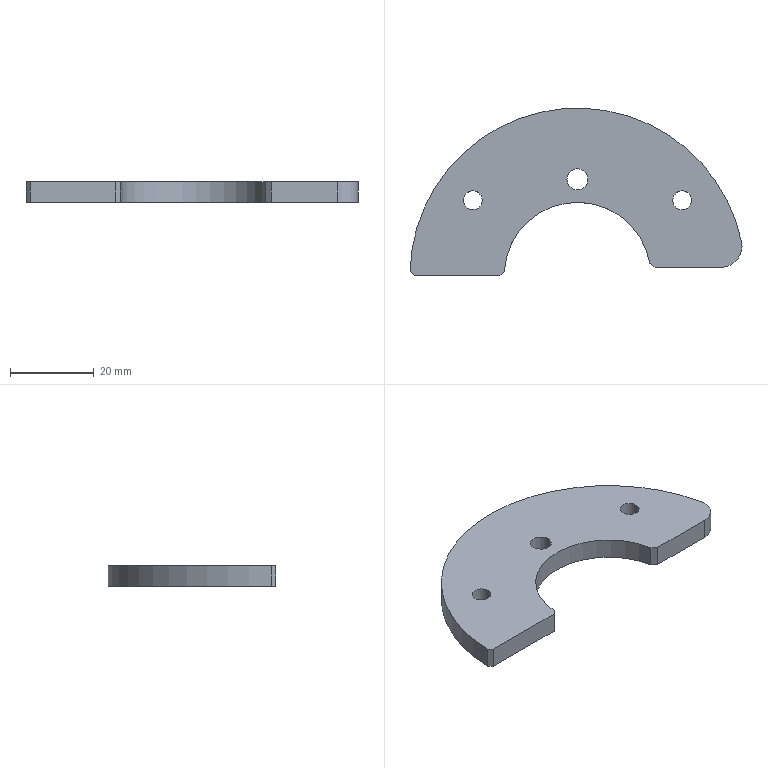Part | STEP file | End cover plate-upper | 1 solid | 16 faces | box 79.281 x 40 x 5 mm | volume 9633 mm3 | cylinder 9 | plane 7 | commonest cylinder face diameters 4.5 x4 5 x2 10 x1 35 x1 80 x1
STEP:
#1=CARTESIAN_POINT('',(0.,0.,0.));
#2=DIRECTION('',(0.,0.,1.));
#3=DIRECTION('',(1.,0.,0.));
#4=AXIS2_PLACEMENT_3D('',#1,#2,#3);
#5=CARTESIAN_POINT('',(-22.75,18.,0.));
#6=VERTEX_POINT('',#5);
#7=CARTESIAN_POINT('',(-22.75,18.,5.));
#8=VERTEX_POINT('',#7);
#9=CARTESIAN_POINT('',(-22.75,18.,5.));
#10=DIRECTION('',(0.,0.,1.));
#11=VECTOR('',#10,1.);
#12=LINE('',#9,#11);
#13=CARTESIAN_POINT('',(-25.,18.,5.));
#14=DIRECTION('',(0.,0.,1.));
#15=DIRECTION('',(1.,0.,0.));
#16=AXIS2_PLACEMENT_3D('',#13,#14,#15);
#17=CYLINDRICAL_SURFACE('',#16,2.25);
#18=CARTESIAN_POINT('',(6.283,0.));
#19=DIRECTION('',(0.,1.));
#20=VECTOR('',#19,1.);
#21=LINE('',#18,#20);
#22=(GEOMETRIC_REPRESENTATION_CONTEXT(2)PARAMETRIC_REPRESENTATION_CONTEXT()REPRESENTATION_CONTEXT('',''));
#23=DEFINITIONAL_REPRESENTATION('',(#21),#22);
#24=PCURVE('',#17,#23);
#25=CARTESIAN_POINT('',(-25.,18.,5.));
#26=DIRECTION('',(0.,0.,1.));
#27=DIRECTION('',(1.,0.,0.));
#28=AXIS2_PLACEMENT_3D('',#25,#26,#27);
#29=CYLINDRICAL_SURFACE('',#28,2.25);
#30=CARTESIAN_POINT('',(0.,0.));
#31=DIRECTION('',(0.,1.));
#32=VECTOR('',#31,1.);
#33=LINE('',#30,#32);
#34=(GEOMETRIC_REPRESENTATION_CONTEXT(2)PARAMETRIC_REPRESENTATION_CONTEXT()REPRESENTATION_CONTEXT('',''));
#35=DEFINITIONAL_REPRESENTATION('',(#33),#34);
#36=PCURVE('',#29,#35);
#37=SURFACE_CURVE('',#12,(#24,#36),.PCURVE_S1.);
#38=EDGE_CURVE('',#6,#8,#37,.T.);
#39=ORIENTED_EDGE('',*,*,#38,.T.);
#40=CARTESIAN_POINT('',(-27.25,18.,5.));
#41=VERTEX_POINT('',#40);
#42=CARTESIAN_POINT('',(-25.,18.,5.));
#43=DIRECTION('',(0.,0.,1.));
#44=DIRECTION('',(1.,0.,0.));
#45=AXIS2_PLACEMENT_3D('',#42,#43,#44);
#46=CIRCLE('',#45,2.25);
#47=CARTESIAN_POINT('',(0.,0.));
#48=DIRECTION('',(1.,0.));
#49=VECTOR('',#48,1.);
#50=LINE('',#47,#49);
#51=(GEOMETRIC_REPRESENTATION_CONTEXT(2)PARAMETRIC_REPRESENTATION_CONTEXT()REPRESENTATION_CONTEXT('',''));
#52=DEFINITIONAL_REPRESENTATION('',(#50),#51);
#53=PCURVE('',#17,#52);
#54=CARTESIAN_POINT('',(0.,0.,5.));
#55=DIRECTION('',(0.,0.,1.));
#56=DIRECTION('',(1.,0.,0.));
#57=AXIS2_PLACEMENT_3D('',#54,#55,#56);
#58=PLANE('',#57);
#59=CARTESIAN_POINT('',(-25.,18.));
#60=DIRECTION('',(1.,0.));
#61=AXIS2_PLACEMENT_2D('',#59,#60);
#62=CIRCLE('',#61,2.25);
#63=(GEOMETRIC_REPRESENTATION_CONTEXT(2)PARAMETRIC_REPRESENTATION_CONTEXT()REPRESENTATION_CONTEXT('',''));
#64=DEFINITIONAL_REPRESENTATION('',(#62),#63);
#65=PCURVE('',#58,#64);
#66=SURFACE_CURVE('',#46,(#53,#65),.PCURVE_S1.);
#67=EDGE_CURVE('',#41,#8,#66,.T.);
#68=ORIENTED_EDGE('',*,*,#67,.F.);
#69=CARTESIAN_POINT('',(-27.25,18.,0.));
#70=VERTEX_POINT('',#69);
#71=CARTESIAN_POINT('',(-27.25,18.,5.));
#72=DIRECTION('',(0.,0.,1.));
#73=VECTOR('',#72,1.);
#74=LINE('',#71,#73);
#75=CARTESIAN_POINT('',(3.142,0.));
#76=DIRECTION('',(0.,1.));
#77=VECTOR('',#76,1.);
#78=LINE('',#75,#77);
#79=(GEOMETRIC_REPRESENTATION_CONTEXT(2)PARAMETRIC_REPRESENTATION_CONTEXT()REPRESENTATION_CONTEXT('',''));
#80=DEFINITIONAL_REPRESENTATION('',(#78),#79);
#81=PCURVE('',#17,#80);
#82=CARTESIAN_POINT('',(3.142,0.));
#83=DIRECTION('',(0.,1.));
#84=VECTOR('',#83,1.);
#85=LINE('',#82,#84);
#86=(GEOMETRIC_REPRESENTATION_CONTEXT(2)PARAMETRIC_REPRESENTATION_CONTEXT()REPRESENTATION_CONTEXT('',''));
#87=DEFINITIONAL_REPRESENTATION('',(#85),#86);
#88=PCURVE('',#29,#87);
#89=SURFACE_CURVE('',#74,(#81,#88),.PCURVE_S1.);
#90=EDGE_CURVE('',#70,#41,#89,.T.);
#91=ORIENTED_EDGE('',*,*,#90,.F.);
#92=CARTESIAN_POINT('',(-25.,18.,0.));
#93=DIRECTION('',(0.,0.,1.));
#94=DIRECTION('',(1.,0.,0.));
#95=AXIS2_PLACEMENT_3D('',#92,#93,#94);
#96=CIRCLE('',#95,2.25);
#97=CARTESIAN_POINT('',(0.,-5.));
#98=DIRECTION('',(1.,0.));
#99=VECTOR('',#98,1.);
#100=LINE('',#97,#99);
#101=(GEOMETRIC_REPRESENTATION_CONTEXT(2)PARAMETRIC_REPRESENTATION_CONTEXT()REPRESENTATION_CONTEXT('',''));
#102=DEFINITIONAL_REPRESENTATION('',(#100),#101);
#103=PCURVE('',#17,#102);
#104=CARTESIAN_POINT('',(0.,0.,0.));
#105=DIRECTION('',(0.,0.,1.));
#106=DIRECTION('',(1.,0.,0.));
#107=AXIS2_PLACEMENT_3D('',#104,#105,#106);
#108=PLANE('',#107);
#109=CARTESIAN_POINT('',(-25.,18.));
#110=DIRECTION('',(1.,0.));
#111=AXIS2_PLACEMENT_2D('',#109,#110);
#112=CIRCLE('',#111,2.25);
#113=(GEOMETRIC_REPRESENTATION_CONTEXT(2)PARAMETRIC_REPRESENTATION_CONTEXT()REPRESENTATION_CONTEXT('',''));
#114=DEFINITIONAL_REPRESENTATION('',(#112),#113);
#115=PCURVE('',#108,#114);
#116=SURFACE_CURVE('',#96,(#103,#115),.PCURVE_S1.);
#117=EDGE_CURVE('',#70,#6,#116,.T.);
#118=ORIENTED_EDGE('',*,*,#117,.T.);
#119=EDGE_LOOP('',(#39,#68,#91,#118));
#120=FACE_BOUND('',#119,.F.);
#121=ADVANCED_FACE('',(#120),#17,.F.);
#122=CARTESIAN_POINT('',(27.25,18.,0.));
#123=VERTEX_POINT('',#122);
#124=CARTESIAN_POINT('',(27.25,18.,5.));
#125=VERTEX_POINT('',#124);
#126=CARTESIAN_POINT('',(27.25,18.,5.));
#127=DIRECTION('',(0.,0.,1.));
#128=VECTOR('',#127,1.);
#129=LINE('',#126,#128);
#130=CARTESIAN_POINT('',(25.,18.,5.));
#131=DIRECTION('',(0.,0.,1.));
#132=DIRECTION('',(1.,0.,0.));
#133=AXIS2_PLACEMENT_3D('',#130,#131,#132);
#134=CYLINDRICAL_SURFACE('',#133,2.25);
#135=CARTESIAN_POINT('',(6.283,0.));
#136=DIRECTION('',(0.,1.));
#137=VECTOR('',#136,1.);
#138=LINE('',#135,#137);
#139=(GEOMETRIC_REPRESENTATION_CONTEXT(2)PARAMETRIC_REPRESENTATION_CONTEXT()REPRESENTATION_CONTEXT('',''));
#140=DEFINITIONAL_REPRESENTATION('',(#138),#139);
#141=PCURVE('',#134,#140);
#142=CARTESIAN_POINT('',(25.,18.,5.));
#143=DIRECTION('',(0.,0.,1.));
#144=DIRECTION('',(1.,0.,0.));
#145=AXIS2_PLACEMENT_3D('',#142,#143,#144);
#146=CYLINDRICAL_SURFACE('',#145,2.25);
#147=CARTESIAN_POINT('',(0.,0.));
#148=DIRECTION('',(0.,1.));
#149=VECTOR('',#148,1.);
#150=LINE('',#147,#149);
#151=(GEOMETRIC_REPRESENTATION_CONTEXT(2)PARAMETRIC_REPRESENTATION_CONTEXT()REPRESENTATION_CONTEXT('',''));
#152=DEFINITIONAL_REPRESENTATION('',(#150),#151);
#153=PCURVE('',#146,#152);
#154=SURFACE_CURVE('',#129,(#141,#153),.PCURVE_S1.);
#155=EDGE_CURVE('',#123,#125,#154,.T.);
#156=ORIENTED_EDGE('',*,*,#155,.T.);
#157=CARTESIAN_POINT('',(22.75,18.,5.));
#158=VERTEX_POINT('',#157);
#159=CARTESIAN_POINT('',(25.,18.,5.));
#160=DIRECTION('',(0.,0.,1.));
#161=DIRECTION('',(1.,0.,0.));
#162=AXIS2_PLACEMENT_3D('',#159,#160,#161);
#163=CIRCLE('',#162,2.25);
#164=CARTESIAN_POINT('',(0.,0.));
#165=DIRECTION('',(1.,0.));
#166=VECTOR('',#165,1.);
#167=LINE('',#164,#166);
#168=(GEOMETRIC_REPRESENTATION_CONTEXT(2)PARAMETRIC_REPRESENTATION_CONTEXT()REPRESENTATION_CONTEXT('',''));
#169=DEFINITIONAL_REPRESENTATION('',(#167),#168);
#170=PCURVE('',#134,#169);
#171=CARTESIAN_POINT('',(25.,18.));
#172=DIRECTION('',(1.,0.));
#173=AXIS2_PLACEMENT_2D('',#171,#172);
#174=CIRCLE('',#173,2.25);
#175=(GEOMETRIC_REPRESENTATION_CONTEXT(2)PARAMETRIC_REPRESENTATION_CONTEXT()REPRESENTATION_CONTEXT('',''));
#176=DEFINITIONAL_REPRESENTATION('',(#174),#175);
#177=PCURVE('',#58,#176);
#178=SURFACE_CURVE('',#163,(#170,#177),.PCURVE_S1.);
#179=EDGE_CURVE('',#158,#125,#178,.T.);
#180=ORIENTED_EDGE('',*,*,#179,.F.);
#181=CARTESIAN_POINT('',(22.75,18.,0.));
#182=VERTEX_POINT('',#181);
#183=CARTESIAN_POINT('',(22.75,18.,5.));
#184=DIRECTION('',(0.,0.,1.));
#185=VECTOR('',#184,1.);
#186=LINE('',#183,#185);
#187=CARTESIAN_POINT('',(3.142,0.));
#188=DIRECTION('',(0.,1.));
#189=VECTOR('',#188,1.);
#190=LINE('',#187,#189);
#191=(GEOMETRIC_REPRESENTATION_CONTEXT(2)PARAMETRIC_REPRESENTATION_CONTEXT()REPRESENTATION_CONTEXT('',''));
#192=DEFINITIONAL_REPRESENTATION('',(#190),#191);
#193=PCURVE('',#134,#192);
#194=CARTESIAN_POINT('',(3.142,0.));
#195=DIRECTION('',(0.,1.));
#196=VECTOR('',#195,1.);
#197=LINE('',#194,#196);
#198=(GEOMETRIC_REPRESENTATION_CONTEXT(2)PARAMETRIC_REPRESENTATION_CONTEXT()REPRESENTATION_CONTEXT('',''));
#199=DEFINITIONAL_REPRESENTATION('',(#197),#198);
#200=PCURVE('',#146,#199);
#201=SURFACE_CURVE('',#186,(#193,#200),.PCURVE_S1.);
#202=EDGE_CURVE('',#182,#158,#201,.T.);
#203=ORIENTED_EDGE('',*,*,#202,.F.);
#204=CARTESIAN_POINT('',(25.,18.,0.));
#205=DIRECTION('',(0.,0.,1.));
#206=DIRECTION('',(1.,0.,0.));
#207=AXIS2_PLACEMENT_3D('',#204,#205,#206);
#208=CIRCLE('',#207,2.25);
#209=CARTESIAN_POINT('',(0.,-5.));
#210=DIRECTION('',(1.,0.));
#211=VECTOR('',#210,1.);
#212=LINE('',#209,#211);
#213=(GEOMETRIC_REPRESENTATION_CONTEXT(2)PARAMETRIC_REPRESENTATION_CONTEXT()REPRESENTATION_CONTEXT('',''));
#214=DEFINITIONAL_REPRESENTATION('',(#212),#213);
#215=PCURVE('',#134,#214);
#216=CARTESIAN_POINT('',(25.,18.));
#217=DIRECTION('',(1.,0.));
#218=AXIS2_PLACEMENT_2D('',#216,#217);
#219=CIRCLE('',#218,2.25);
#220=(GEOMETRIC_REPRESENTATION_CONTEXT(2)PARAMETRIC_REPRESENTATION_CONTEXT()REPRESENTATION_CONTEXT('',''));
#221=DEFINITIONAL_REPRESENTATION('',(#219),#220);
#222=PCURVE('',#108,#221);
#223=SURFACE_CURVE('',#208,(#215,#222),.PCURVE_S1.);
#224=EDGE_CURVE('',#182,#123,#223,.T.);
#225=ORIENTED_EDGE('',*,*,#224,.T.);
#226=EDGE_LOOP('',(#156,#180,#203,#225));
#227=FACE_BOUND('',#226,.F.);
#228=ADVANCED_FACE('',(#227),#134,.F.);
#229=CARTESIAN_POINT('',(2.5,23.,0.));
#230=VERTEX_POINT('',#229);
#231=CARTESIAN_POINT('',(2.5,23.,5.));
#232=VERTEX_POINT('',#231);
#233=CARTESIAN_POINT('',(2.5,23.,5.));
#234=DIRECTION('',(0.,0.,1.));
#235=VECTOR('',#234,1.);
#236=LINE('',#233,#235);
#237=CARTESIAN_POINT('',(0.,23.,5.));
#238=DIRECTION('',(0.,0.,1.));
#239=DIRECTION('',(1.,0.,0.));
#240=AXIS2_PLACEMENT_3D('',#237,#238,#239);
#241=CYLINDRICAL_SURFACE('',#240,2.5);
#242=CARTESIAN_POINT('',(6.283,0.));
#243=DIRECTION('',(0.,1.));
#244=VECTOR('',#243,1.);
#245=LINE('',#242,#244);
#246=(GEOMETRIC_REPRESENTATION_CONTEXT(2)PARAMETRIC_REPRESENTATION_CONTEXT()REPRESENTATION_CONTEXT('',''));
#247=DEFINITIONAL_REPRESENTATION('',(#245),#246);
#248=PCURVE('',#241,#247);
#249=CARTESIAN_POINT('',(0.,23.,5.));
#250=DIRECTION('',(0.,0.,1.));
#251=DIRECTION('',(1.,0.,0.));
#252=AXIS2_PLACEMENT_3D('',#249,#250,#251);
#253=CYLINDRICAL_SURFACE('',#252,2.5);
#254=CARTESIAN_POINT('',(0.,0.));
#255=DIRECTION('',(0.,1.));
#256=VECTOR('',#255,1.);
#257=LINE('',#254,#256);
#258=(GEOMETRIC_REPRESENTATION_CONTEXT(2)PARAMETRIC_REPRESENTATION_CONTEXT()REPRESENTATION_CONTEXT('',''));
#259=DEFINITIONAL_REPRESENTATION('',(#257),#258);
#260=PCURVE('',#253,#259);
#261=SURFACE_CURVE('',#236,(#248,#260),.PCURVE_S1.);
#262=EDGE_CURVE('',#230,#232,#261,.T.);
#263=ORIENTED_EDGE('',*,*,#262,.T.);
#264=CARTESIAN_POINT('',(-2.5,23.,5.));
#265=VERTEX_POINT('',#264);
#266=CARTESIAN_POINT('',(0.,23.,5.));
#267=DIRECTION('',(0.,0.,1.));
#268=DIRECTION('',(1.,0.,0.));
#269=AXIS2_PLACEMENT_3D('',#266,#267,#268);
#270=CIRCLE('',#269,2.5);
#271=CARTESIAN_POINT('',(0.,0.));
#272=DIRECTION('',(1.,0.));
#273=VECTOR('',#272,1.);
#274=LINE('',#271,#273);
#275=(GEOMETRIC_REPRESENTATION_CONTEXT(2)PARAMETRIC_REPRESENTATION_CONTEXT()REPRESENTATION_CONTEXT('',''));
#276=DEFINITIONAL_REPRESENTATION('',(#274),#275);
#277=PCURVE('',#241,#276);
#278=CARTESIAN_POINT('',(0.,23.));
#279=DIRECTION('',(1.,0.));
#280=AXIS2_PLACEMENT_2D('',#278,#279);
#281=CIRCLE('',#280,2.5);
#282=(GEOMETRIC_REPRESENTATION_CONTEXT(2)PARAMETRIC_REPRESENTATION_CONTEXT()REPRESENTATION_CONTEXT('',''));
#283=DEFINITIONAL_REPRESENTATION('',(#281),#282);
#284=PCURVE('',#58,#283);
#285=SURFACE_CURVE('',#270,(#277,#284),.PCURVE_S1.);
#286=EDGE_CURVE('',#265,#232,#285,.T.);
#287=ORIENTED_EDGE('',*,*,#286,.F.);
#288=CARTESIAN_POINT('',(-2.5,23.,0.));
#289=VERTEX_POINT('',#288);
#290=CARTESIAN_POINT('',(-2.5,23.,5.));
#291=DIRECTION('',(0.,0.,1.));
#292=VECTOR('',#291,1.);
#293=LINE('',#290,#292);
#294=CARTESIAN_POINT('',(3.142,0.));
#295=DIRECTION('',(0.,1.));
#296=VECTOR('',#295,1.);
#297=LINE('',#294,#296);
#298=(GEOMETRIC_REPRESENTATION_CONTEXT(2)PARAMETRIC_REPRESENTATION_CONTEXT()REPRESENTATION_CONTEXT('',''));
#299=DEFINITIONAL_REPRESENTATION('',(#297),#298);
#300=PCURVE('',#241,#299);
#301=CARTESIAN_POINT('',(3.142,0.));
#302=DIRECTION('',(0.,1.));
#303=VECTOR('',#302,1.);
#304=LINE('',#301,#303);
#305=(GEOMETRIC_REPRESENTATION_CONTEXT(2)PARAMETRIC_REPRESENTATION_CONTEXT()REPRESENTATION_CONTEXT('',''));
#306=DEFINITIONAL_REPRESENTATION('',(#304),#305);
#307=PCURVE('',#253,#306);
#308=SURFACE_CURVE('',#293,(#300,#307),.PCURVE_S1.);
#309=EDGE_CURVE('',#289,#265,#308,.T.);
#310=ORIENTED_EDGE('',*,*,#309,.F.);
#311=CARTESIAN_POINT('',(0.,23.,0.));
#312=DIRECTION('',(0.,0.,1.));
#313=DIRECTION('',(1.,0.,0.));
#314=AXIS2_PLACEMENT_3D('',#311,#312,#313);
#315=CIRCLE('',#314,2.5);
#316=CARTESIAN_POINT('',(0.,-5.));
#317=DIRECTION('',(1.,0.));
#318=VECTOR('',#317,1.);
#319=LINE('',#316,#318);
#320=(GEOMETRIC_REPRESENTATION_CONTEXT(2)PARAMETRIC_REPRESENTATION_CONTEXT()REPRESENTATION_CONTEXT('',''));
#321=DEFINITIONAL_REPRESENTATION('',(#319),#320);
#322=PCURVE('',#241,#321);
#323=CARTESIAN_POINT('',(0.,23.));
#324=DIRECTION('',(1.,0.));
#325=AXIS2_PLACEMENT_2D('',#323,#324);
#326=CIRCLE('',#325,2.5);
#327=(GEOMETRIC_REPRESENTATION_CONTEXT(2)PARAMETRIC_REPRESENTATION_CONTEXT()REPRESENTATION_CONTEXT('',''));
#328=DEFINITIONAL_REPRESENTATION('',(#326),#327);
#329=PCURVE('',#108,#328);
#330=SURFACE_CURVE('',#315,(#322,#329),.PCURVE_S1.);
#331=EDGE_CURVE('',#289,#230,#330,.T.);
#332=ORIENTED_EDGE('',*,*,#331,.T.);
#333=EDGE_LOOP('',(#263,#287,#310,#332));
#334=FACE_BOUND('',#333,.F.);
#335=ADVANCED_FACE('',(#334),#241,.F.);
#336=CARTESIAN_POINT('',(-25.,18.,5.));
#337=DIRECTION('',(0.,0.,1.));
#338=DIRECTION('',(1.,0.,0.));
#339=AXIS2_PLACEMENT_3D('',#336,#337,#338);
#340=CIRCLE('',#339,2.25);
#341=CARTESIAN_POINT('',(-25.,18.));
#342=DIRECTION('',(1.,0.));
#343=AXIS2_PLACEMENT_2D('',#341,#342);
#344=CIRCLE('',#343,2.25);
#345=(GEOMETRIC_REPRESENTATION_CONTEXT(2)PARAMETRIC_REPRESENTATION_CONTEXT()REPRESENTATION_CONTEXT('',''));
#346=DEFINITIONAL_REPRESENTATION('',(#344),#345);
#347=PCURVE('',#58,#346);
#348=CARTESIAN_POINT('',(0.,0.));
#349=DIRECTION('',(1.,0.));
#350=VECTOR('',#349,1.);
#351=LINE('',#348,#350);
#352=(GEOMETRIC_REPRESENTATION_CONTEXT(2)PARAMETRIC_REPRESENTATION_CONTEXT()REPRESENTATION_CONTEXT('',''));
#353=DEFINITIONAL_REPRESENTATION('',(#351),#352);
#354=PCURVE('',#29,#353);
#355=SURFACE_CURVE('',#340,(#347,#354),.PCURVE_S1.);
#356=EDGE_CURVE('',#8,#41,#355,.T.);
#357=ORIENTED_EDGE('',*,*,#356,.F.);
#358=ORIENTED_EDGE('',*,*,#67,.F.);
#359=EDGE_LOOP('',(#357,#358));
#360=FACE_BOUND('',#359,.T.);
#361=CARTESIAN_POINT('',(25.,18.,5.));
#362=DIRECTION('',(0.,0.,1.));
#363=DIRECTION('',(1.,0.,0.));
#364=AXIS2_PLACEMENT_3D('',#361,#362,#363);
#365=CIRCLE('',#364,2.25);
#366=CARTESIAN_POINT('',(25.,18.));
#367=DIRECTION('',(1.,0.));
#368=AXIS2_PLACEMENT_2D('',#366,#367);
#369=CIRCLE('',#368,2.25);
#370=(GEOMETRIC_REPRESENTATION_CONTEXT(2)PARAMETRIC_REPRESENTATION_CONTEXT()REPRESENTATION_CONTEXT('',''));
#371=DEFINITIONAL_REPRESENTATION('',(#369),#370);
#372=PCURVE('',#58,#371);
#373=CARTESIAN_POINT('',(0.,0.));
#374=DIRECTION('',(1.,0.));
#375=VECTOR('',#374,1.);
#376=LINE('',#373,#375);
#377=(GEOMETRIC_REPRESENTATION_CONTEXT(2)PARAMETRIC_REPRESENTATION_CONTEXT()REPRESENTATION_CONTEXT('',''));
#378=DEFINITIONAL_REPRESENTATION('',(#376),#377);
#379=PCURVE('',#146,#378);
#380=SURFACE_CURVE('',#365,(#372,#379),.PCURVE_S1.);
#381=EDGE_CURVE('',#125,#158,#380,.T.);
#382=ORIENTED_EDGE('',*,*,#381,.F.);
#383=ORIENTED_EDGE('',*,*,#179,.F.);
#384=EDGE_LOOP('',(#382,#383));
#385=FACE_BOUND('',#384,.T.);
#386=CARTESIAN_POINT('',(17.237,3.02,5.));
#387=VERTEX_POINT('',#386);
#388=CARTESIAN_POINT('',(-17.47,1.03,5.));
#389=VERTEX_POINT('',#388);
#390=CARTESIAN_POINT('',(0.,0.,5.));
#391=DIRECTION('',(0.,0.,1.));
#392=DIRECTION('',(1.,0.,0.));
#393=AXIS2_PLACEMENT_3D('',#390,#391,#392);
#394=CIRCLE('',#393,17.5);
#395=CARTESIAN_POINT('',(0.,0.));
#396=DIRECTION('',(1.,0.));
#397=AXIS2_PLACEMENT_2D('',#395,#396);
#398=CIRCLE('',#397,17.5);
#399=(GEOMETRIC_REPRESENTATION_CONTEXT(2)PARAMETRIC_REPRESENTATION_CONTEXT()REPRESENTATION_CONTEXT('',''));
#400=DEFINITIONAL_REPRESENTATION('',(#398),#399);
#401=PCURVE('',#58,#400);
#402=CARTESIAN_POINT('',(0.,0.,5.));
#403=DIRECTION('',(0.,0.,-1.));
#404=DIRECTION('',(-1.,0.,0.));
#405=AXIS2_PLACEMENT_3D('',#402,#403,#404);
#406=CYLINDRICAL_SURFACE('',#405,17.5);
#407=CARTESIAN_POINT('',(3.142,0.));
#408=DIRECTION('',(-1.,0.));
#409=VECTOR('',#408,1.);
#410=LINE('',#407,#409);
#411=(GEOMETRIC_REPRESENTATION_CONTEXT(2)PARAMETRIC_REPRESENTATION_CONTEXT()REPRESENTATION_CONTEXT('',''));
#412=DEFINITIONAL_REPRESENTATION('',(#410),#411);
#413=PCURVE('',#406,#412);
#414=SURFACE_CURVE('',#394,(#401,#413),.PCURVE_S1.);
#415=EDGE_CURVE('',#387,#389,#414,.T.);
#416=ORIENTED_EDGE('',*,*,#415,.F.);
#417=CARTESIAN_POINT('',(18.523,2.,5.));
#418=VERTEX_POINT('',#417);
#419=CARTESIAN_POINT('',(8.132,10.247,5.));
#420=DIRECTION('',(0.7833,-0.6217,0.));
#421=VECTOR('',#420,1.);
#422=LINE('',#419,#421);
#423=CARTESIAN_POINT('',(8.132,10.247));
#424=DIRECTION('',(0.7833,-0.6217));
#425=VECTOR('',#424,1.);
#426=LINE('',#423,#425);
#427=(GEOMETRIC_REPRESENTATION_CONTEXT(2)PARAMETRIC_REPRESENTATION_CONTEXT()REPRESENTATION_CONTEXT('',''));
#428=DEFINITIONAL_REPRESENTATION('',(#426),#427);
#429=PCURVE('',#58,#428);
#430=CARTESIAN_POINT('',(18.523,2.,5.));
#431=DIRECTION('',(0.6217,0.7833,0.));
#432=DIRECTION('',(0.,0.,-1.));
#433=AXIS2_PLACEMENT_3D('',#430,#431,#432);
#434=PLANE('',#433);
#435=CARTESIAN_POINT('',(0.,13.265));
#436=DIRECTION('',(0.,-1.));
#437=VECTOR('',#436,1.);
#438=LINE('',#435,#437);
#439=(GEOMETRIC_REPRESENTATION_CONTEXT(2)PARAMETRIC_REPRESENTATION_CONTEXT()REPRESENTATION_CONTEXT('',''));
#440=DEFINITIONAL_REPRESENTATION('',(#438),#439);
#441=PCURVE('',#434,#440);
#442=SURFACE_CURVE('',#422,(#429,#441),.PCURVE_S1.);
#443=EDGE_CURVE('',#387,#418,#442,.T.);
#444=ORIENTED_EDGE('',*,*,#443,.T.);
#445=CARTESIAN_POINT('',(34.293,2.,5.));
#446=VERTEX_POINT('',#445);
#447=CARTESIAN_POINT('',(12.976,2.,5.));
#448=DIRECTION('',(-1.,0.,0.));
#449=VECTOR('',#448,1.);
#450=LINE('',#447,#449);
#451=CARTESIAN_POINT('',(12.976,2.));
#452=DIRECTION('',(-1.,0.));
#453=VECTOR('',#452,1.);
#454=LINE('',#451,#453);
#455=(GEOMETRIC_REPRESENTATION_CONTEXT(2)PARAMETRIC_REPRESENTATION_CONTEXT()REPRESENTATION_CONTEXT('',''));
#456=DEFINITIONAL_REPRESENTATION('',(#454),#455);
#457=PCURVE('',#58,#456);
#458=CARTESIAN_POINT('',(12.976,2.,0.));
#459=DIRECTION('',(0.,1.,0.));
#460=DIRECTION('',(0.,0.,1.));
#461=AXIS2_PLACEMENT_3D('',#458,#459,#460);
#462=PLANE('',#461);
#463=CARTESIAN_POINT('',(5.,0.));
#464=DIRECTION('',(0.,-1.));
#465=VECTOR('',#464,1.);
#466=LINE('',#463,#465);
#467=(GEOMETRIC_REPRESENTATION_CONTEXT(2)PARAMETRIC_REPRESENTATION_CONTEXT()REPRESENTATION_CONTEXT('',''));
#468=DEFINITIONAL_REPRESENTATION('',(#466),#467);
#469=PCURVE('',#462,#468);
#470=SURFACE_CURVE('',#450,(#457,#469),.PCURVE_S1.);
#471=EDGE_CURVE('',#446,#418,#470,.T.);
#472=ORIENTED_EDGE('',*,*,#471,.F.);
#473=CARTESIAN_POINT('',(39.192,8.,5.));
#474=VERTEX_POINT('',#473);
#475=CARTESIAN_POINT('',(34.293,7.,5.));
#476=DIRECTION('',(0.,0.,1.));
#477=DIRECTION('',(1.,0.,0.));
#478=AXIS2_PLACEMENT_3D('',#475,#476,#477);
#479=CIRCLE('',#478,5.);
#480=CARTESIAN_POINT('',(34.293,7.));
#481=DIRECTION('',(1.,0.));
#482=AXIS2_PLACEMENT_2D('',#480,#481);
#483=CIRCLE('',#482,5.);
#484=(GEOMETRIC_REPRESENTATION_CONTEXT(2)PARAMETRIC_REPRESENTATION_CONTEXT()REPRESENTATION_CONTEXT('',''));
#485=DEFINITIONAL_REPRESENTATION('',(#483),#484);
#486=PCURVE('',#58,#485);
#487=CARTESIAN_POINT('',(34.293,7.,5.));
#488=DIRECTION('',(0.,0.,-1.));
#489=DIRECTION('',(-1.,0.,0.));
#490=AXIS2_PLACEMENT_3D('',#487,#488,#489);
#491=CYLINDRICAL_SURFACE('',#490,5.);
#492=CARTESIAN_POINT('',(9.425,0.));
#493=DIRECTION('',(-1.,0.));
#494=VECTOR('',#493,1.);
#495=LINE('',#492,#494);
#496=(GEOMETRIC_REPRESENTATION_CONTEXT(2)PARAMETRIC_REPRESENTATION_CONTEXT()REPRESENTATION_CONTEXT('',''));
#497=DEFINITIONAL_REPRESENTATION('',(#495),#496);
#498=PCURVE('',#491,#497);
#499=SURFACE_CURVE('',#479,(#486,#498),.PCURVE_S1.);
#500=EDGE_CURVE('',#446,#474,#499,.T.);
#501=ORIENTED_EDGE('',*,*,#500,.T.);
#502=CARTESIAN_POINT('',(-39.988,0.9878,5.));
#503=VERTEX_POINT('',#502);
#504=CARTESIAN_POINT('',(0.,0.,5.));
#505=DIRECTION('',(0.,0.,1.));
#506=DIRECTION('',(1.,0.,0.));
#507=AXIS2_PLACEMENT_3D('',#504,#505,#506);
#508=CIRCLE('',#507,40.);
#509=CARTESIAN_POINT('',(0.,0.));
#510=DIRECTION('',(1.,0.));
#511=AXIS2_PLACEMENT_2D('',#509,#510);
#512=CIRCLE('',#511,40.);
#513=(GEOMETRIC_REPRESENTATION_CONTEXT(2)PARAMETRIC_REPRESENTATION_CONTEXT()REPRESENTATION_CONTEXT('',''));
#514=DEFINITIONAL_REPRESENTATION('',(#512),#513);
#515=PCURVE('',#58,#514);
#516=CARTESIAN_POINT('',(0.,0.,5.));
#517=DIRECTION('',(0.,0.,-1.));
#518=DIRECTION('',(-1.,0.,0.));
#519=AXIS2_PLACEMENT_3D('',#516,#517,#518);
#520=CYLINDRICAL_SURFACE('',#519,40.);
#521=CARTESIAN_POINT('',(3.142,0.));
#522=DIRECTION('',(-1.,0.));
#523=VECTOR('',#522,1.);
#524=LINE('',#521,#523);
#525=(GEOMETRIC_REPRESENTATION_CONTEXT(2)PARAMETRIC_REPRESENTATION_CONTEXT()REPRESENTATION_CONTEXT('',''));
#526=DEFINITIONAL_REPRESENTATION('',(#524),#525);
#527=PCURVE('',#520,#526);
#528=SURFACE_CURVE('',#508,(#515,#527),.PCURVE_S1.);
#529=EDGE_CURVE('',#474,#503,#528,.T.);
#530=ORIENTED_EDGE('',*,*,#529,.T.);
#531=CARTESIAN_POINT('',(-39.,0.,5.));
#532=VERTEX_POINT('',#531);
#533=CARTESIAN_POINT('',(-19.5,-19.5,5.));
#534=DIRECTION('',(0.7071,-0.7071,0.));
#535=VECTOR('',#534,1.);
#536=LINE('',#533,#535);
#537=CARTESIAN_POINT('',(-19.5,-19.5));
#538=DIRECTION('',(0.7071,-0.7071));
#539=VECTOR('',#538,1.);
#540=LINE('',#537,#539);
#541=(GEOMETRIC_REPRESENTATION_CONTEXT(2)PARAMETRIC_REPRESENTATION_CONTEXT()REPRESENTATION_CONTEXT('',''));
#542=DEFINITIONAL_REPRESENTATION('',(#540),#541);
#543=PCURVE('',#58,#542);
#544=CARTESIAN_POINT('',(-39.988,0.9878,5.));
#545=DIRECTION('',(-0.7071,-0.7071,0.));
#546=DIRECTION('',(0.,0.,-1.));
#547=AXIS2_PLACEMENT_3D('',#544,#545,#546);
#548=PLANE('',#547);
#549=CARTESIAN_POINT('',(0.,28.974));
#550=DIRECTION('',(0.,1.));
#551=VECTOR('',#550,1.);
#552=LINE('',#549,#551);
#553=(GEOMETRIC_REPRESENTATION_CONTEXT(2)PARAMETRIC_REPRESENTATION_CONTEXT()REPRESENTATION_CONTEXT('',''));
#554=DEFINITIONAL_REPRESENTATION('',(#552),#553);
#555=PCURVE('',#548,#554);
#556=SURFACE_CURVE('',#536,(#543,#555),.PCURVE_S1.);
#557=EDGE_CURVE('',#503,#532,#556,.T.);
#558=ORIENTED_EDGE('',*,*,#557,.T.);
#559=CARTESIAN_POINT('',(-18.5,0.,5.));
#560=VERTEX_POINT('',#559);
#561=CARTESIAN_POINT('',(-62.088,0.,5.));
#562=DIRECTION('',(-1.,0.,0.));
#563=VECTOR('',#562,1.);
#564=LINE('',#561,#563);
#565=CARTESIAN_POINT('',(-62.088,0.));
#566=DIRECTION('',(-1.,0.));
#567=VECTOR('',#566,1.);
#568=LINE('',#565,#567);
#569=(GEOMETRIC_REPRESENTATION_CONTEXT(2)PARAMETRIC_REPRESENTATION_CONTEXT()REPRESENTATION_CONTEXT('',''));
#570=DEFINITIONAL_REPRESENTATION('',(#568),#569);
#571=PCURVE('',#58,#570);
#572=CARTESIAN_POINT('',(-62.088,0.,0.));
#573=DIRECTION('',(0.,1.,0.));
#574=DIRECTION('',(0.,0.,1.));
#575=AXIS2_PLACEMENT_3D('',#572,#573,#574);
#576=PLANE('',#575);
#577=CARTESIAN_POINT('',(5.,0.));
#578=DIRECTION('',(0.,-1.));
#579=VECTOR('',#578,1.);
#580=LINE('',#577,#579);
#581=(GEOMETRIC_REPRESENTATION_CONTEXT(2)PARAMETRIC_REPRESENTATION_CONTEXT()REPRESENTATION_CONTEXT('',''));
#582=DEFINITIONAL_REPRESENTATION('',(#580),#581);
#583=PCURVE('',#576,#582);
#584=SURFACE_CURVE('',#564,(#571,#583),.PCURVE_S1.);
#585=EDGE_CURVE('',#560,#532,#584,.T.);
#586=ORIENTED_EDGE('',*,*,#585,.F.);
#587=CARTESIAN_POINT('',(-9.25,9.25,5.));
#588=DIRECTION('',(0.7071,0.7071,0.));
#589=VECTOR('',#588,1.);
#590=LINE('',#587,#589);
#591=CARTESIAN_POINT('',(-9.25,9.25));
#592=DIRECTION('',(0.7071,0.7071));
#593=VECTOR('',#592,1.);
#594=LINE('',#591,#593);
#595=(GEOMETRIC_REPRESENTATION_CONTEXT(2)PARAMETRIC_REPRESENTATION_CONTEXT()REPRESENTATION_CONTEXT('',''));
#596=DEFINITIONAL_REPRESENTATION('',(#594),#595);
#597=PCURVE('',#58,#596);
#598=CARTESIAN_POINT('',(-18.5,0.,5.));
#599=DIRECTION('',(0.7071,-0.7071,0.));
#600=DIRECTION('',(0.,0.,-1.));
#601=AXIS2_PLACEMENT_3D('',#598,#599,#600);
#602=PLANE('',#601);
#603=CARTESIAN_POINT('',(0.,13.081));
#604=DIRECTION('',(0.,1.));
#605=VECTOR('',#604,1.);
#606=LINE('',#603,#605);
#607=(GEOMETRIC_REPRESENTATION_CONTEXT(2)PARAMETRIC_REPRESENTATION_CONTEXT()REPRESENTATION_CONTEXT('',''));
#608=DEFINITIONAL_REPRESENTATION('',(#606),#607);
#609=PCURVE('',#602,#608);
#610=SURFACE_CURVE('',#590,(#597,#609),.PCURVE_S1.);
#611=EDGE_CURVE('',#560,#389,#610,.T.);
#612=ORIENTED_EDGE('',*,*,#611,.T.);
#613=EDGE_LOOP('',(#416,#444,#472,#501,#530,#558,#586,#612));
#614=FACE_BOUND('',#613,.T.);
#615=CARTESIAN_POINT('',(0.,23.,5.));
#616=DIRECTION('',(0.,0.,1.));
#617=DIRECTION('',(1.,0.,0.));
#618=AXIS2_PLACEMENT_3D('',#615,#616,#617);
#619=CIRCLE('',#618,2.5);
#620=CARTESIAN_POINT('',(0.,23.));
#621=DIRECTION('',(1.,0.));
#622=AXIS2_PLACEMENT_2D('',#620,#621);
#623=CIRCLE('',#622,2.5);
#624=(GEOMETRIC_REPRESENTATION_CONTEXT(2)PARAMETRIC_REPRESENTATION_CONTEXT()REPRESENTATION_CONTEXT('',''));
#625=DEFINITIONAL_REPRESENTATION('',(#623),#624);
#626=PCURVE('',#58,#625);
#627=CARTESIAN_POINT('',(0.,0.));
#628=DIRECTION('',(1.,0.));
#629=VECTOR('',#628,1.);
#630=LINE('',#627,#629);
#631=(GEOMETRIC_REPRESENTATION_CONTEXT(2)PARAMETRIC_REPRESENTATION_CONTEXT()REPRESENTATION_CONTEXT('',''));
#632=DEFINITIONAL_REPRESENTATION('',(#630),#631);
#633=PCURVE('',#253,#632);
#634=SURFACE_CURVE('',#619,(#626,#633),.PCURVE_S1.);
#635=EDGE_CURVE('',#232,#265,#634,.T.);
#636=ORIENTED_EDGE('',*,*,#635,.F.);
#637=ORIENTED_EDGE('',*,*,#286,.F.);
#638=EDGE_LOOP('',(#636,#637));
#639=FACE_BOUND('',#638,.T.);
#640=ADVANCED_FACE('',(#360,#385,#614,#639),#58,.T.);
#641=CARTESIAN_POINT('',(-25.,18.,0.));
#642=DIRECTION('',(0.,0.,1.));
#643=DIRECTION('',(1.,0.,0.));
#644=AXIS2_PLACEMENT_3D('',#641,#642,#643);
#645=CIRCLE('',#644,2.25);
#646=CARTESIAN_POINT('',(-25.,18.));
#647=DIRECTION('',(1.,0.));
#648=AXIS2_PLACEMENT_2D('',#646,#647);
#649=CIRCLE('',#648,2.25);
#650=(GEOMETRIC_REPRESENTATION_CONTEXT(2)PARAMETRIC_REPRESENTATION_CONTEXT()REPRESENTATION_CONTEXT('',''));
#651=DEFINITIONAL_REPRESENTATION('',(#649),#650);
#652=PCURVE('',#108,#651);
#653=CARTESIAN_POINT('',(0.,-5.));
#654=DIRECTION('',(1.,0.));
#655=VECTOR('',#654,1.);
#656=LINE('',#653,#655);
#657=(GEOMETRIC_REPRESENTATION_CONTEXT(2)PARAMETRIC_REPRESENTATION_CONTEXT()REPRESENTATION_CONTEXT('',''));
#658=DEFINITIONAL_REPRESENTATION('',(#656),#657);
#659=PCURVE('',#29,#658);
#660=SURFACE_CURVE('',#645,(#652,#659),.PCURVE_S1.);
#661=EDGE_CURVE('',#6,#70,#660,.T.);
#662=ORIENTED_EDGE('',*,*,#661,.T.);
#663=ORIENTED_EDGE('',*,*,#117,.T.);
#664=EDGE_LOOP('',(#662,#663));
#665=FACE_BOUND('',#664,.T.);
#666=CARTESIAN_POINT('',(25.,18.,0.));
#667=DIRECTION('',(0.,0.,1.));
#668=DIRECTION('',(1.,0.,0.));
#669=AXIS2_PLACEMENT_3D('',#666,#667,#668);
#670=CIRCLE('',#669,2.25);
#671=CARTESIAN_POINT('',(25.,18.));
#672=DIRECTION('',(1.,0.));
#673=AXIS2_PLACEMENT_2D('',#671,#672);
#674=CIRCLE('',#673,2.25);
#675=(GEOMETRIC_REPRESENTATION_CONTEXT(2)PARAMETRIC_REPRESENTATION_CONTEXT()REPRESENTATION_CONTEXT('',''));
#676=DEFINITIONAL_REPRESENTATION('',(#674),#675);
#677=PCURVE('',#108,#676);
#678=CARTESIAN_POINT('',(0.,-5.));
#679=DIRECTION('',(1.,0.));
#680=VECTOR('',#679,1.);
#681=LINE('',#678,#680);
#682=(GEOMETRIC_REPRESENTATION_CONTEXT(2)PARAMETRIC_REPRESENTATION_CONTEXT()REPRESENTATION_CONTEXT('',''));
#683=DEFINITIONAL_REPRESENTATION('',(#681),#682);
#684=PCURVE('',#146,#683);
#685=SURFACE_CURVE('',#670,(#677,#684),.PCURVE_S1.);
#686=EDGE_CURVE('',#123,#182,#685,.T.);
#687=ORIENTED_EDGE('',*,*,#686,.T.);
#688=ORIENTED_EDGE('',*,*,#224,.T.);
#689=EDGE_LOOP('',(#687,#688));
#690=FACE_BOUND('',#689,.T.);
#691=CARTESIAN_POINT('',(0.,23.,0.));
#692=DIRECTION('',(0.,0.,1.));
#693=DIRECTION('',(1.,0.,0.));
#694=AXIS2_PLACEMENT_3D('',#691,#692,#693);
#695=CIRCLE('',#694,2.5);
#696=CARTESIAN_POINT('',(0.,23.));
#697=DIRECTION('',(1.,0.));
#698=AXIS2_PLACEMENT_2D('',#696,#697);
#699=CIRCLE('',#698,2.5);
#700=(GEOMETRIC_REPRESENTATION_CONTEXT(2)PARAMETRIC_REPRESENTATION_CONTEXT()REPRESENTATION_CONTEXT('',''));
#701=DEFINITIONAL_REPRESENTATION('',(#699),#700);
#702=PCURVE('',#108,#701);
#703=CARTESIAN_POINT('',(0.,-5.));
#704=DIRECTION('',(1.,0.));
#705=VECTOR('',#704,1.);
#706=LINE('',#703,#705);
#707=(GEOMETRIC_REPRESENTATION_CONTEXT(2)PARAMETRIC_REPRESENTATION_CONTEXT()REPRESENTATION_CONTEXT('',''));
#708=DEFINITIONAL_REPRESENTATION('',(#706),#707);
#709=PCURVE('',#253,#708);
#710=SURFACE_CURVE('',#695,(#702,#709),.PCURVE_S1.);
#711=EDGE_CURVE('',#230,#289,#710,.T.);
#712=ORIENTED_EDGE('',*,*,#711,.T.);
#713=ORIENTED_EDGE('',*,*,#331,.T.);
#714=EDGE_LOOP('',(#712,#713));
#715=FACE_BOUND('',#714,.T.);
#716=CARTESIAN_POINT('',(34.293,2.,0.));
#717=VERTEX_POINT('',#716);
#718=CARTESIAN_POINT('',(18.523,2.,0.));
#719=VERTEX_POINT('',#718);
#720=CARTESIAN_POINT('',(12.976,2.,0.));
#721=DIRECTION('',(-1.,0.,0.));
#722=VECTOR('',#721,1.);
#723=LINE('',#720,#722);
#724=CARTESIAN_POINT('',(12.976,2.));
#725=DIRECTION('',(-1.,0.));
#726=VECTOR('',#725,1.);
#727=LINE('',#724,#726);
#728=(GEOMETRIC_REPRESENTATION_CONTEXT(2)PARAMETRIC_REPRESENTATION_CONTEXT()REPRESENTATION_CONTEXT('',''));
#729=DEFINITIONAL_REPRESENTATION('',(#727),#728);
#730=PCURVE('',#108,#729);
#731=CARTESIAN_POINT('',(0.,0.));
#732=DIRECTION('',(0.,-1.));
#733=VECTOR('',#732,1.);
#734=LINE('',#731,#733);
#735=(GEOMETRIC_REPRESENTATION_CONTEXT(2)PARAMETRIC_REPRESENTATION_CONTEXT()REPRESENTATION_CONTEXT('',''));
#736=DEFINITIONAL_REPRESENTATION('',(#734),#735);
#737=PCURVE('',#462,#736);
#738=SURFACE_CURVE('',#723,(#730,#737),.PCURVE_S1.);
#739=EDGE_CURVE('',#717,#719,#738,.T.);
#740=ORIENTED_EDGE('',*,*,#739,.T.);
#741=CARTESIAN_POINT('',(17.237,3.02,0.));
#742=VERTEX_POINT('',#741);
#743=CARTESIAN_POINT('',(18.523,2.,0.));
#744=DIRECTION('',(-0.7833,0.6217,0.));
#745=VECTOR('',#744,1.);
#746=LINE('',#743,#745);
#747=CARTESIAN_POINT('',(18.523,2.));
#748=DIRECTION('',(-0.7833,0.6217));
#749=VECTOR('',#748,1.);
#750=LINE('',#747,#749);
#751=(GEOMETRIC_REPRESENTATION_CONTEXT(2)PARAMETRIC_REPRESENTATION_CONTEXT()REPRESENTATION_CONTEXT('',''));
#752=DEFINITIONAL_REPRESENTATION('',(#750),#751);
#753=PCURVE('',#108,#752);
#754=CARTESIAN_POINT('',(5.,0.));
#755=DIRECTION('',(0.,1.));
#756=VECTOR('',#755,1.);
#757=LINE('',#754,#756);
#758=(GEOMETRIC_REPRESENTATION_CONTEXT(2)PARAMETRIC_REPRESENTATION_CONTEXT()REPRESENTATION_CONTEXT('',''));
#759=DEFINITIONAL_REPRESENTATION('',(#757),#758);
#760=PCURVE('',#434,#759);
#761=SURFACE_CURVE('',#746,(#753,#760),.PCURVE_S1.);
#762=EDGE_CURVE('',#719,#742,#761,.T.);
#763=ORIENTED_EDGE('',*,*,#762,.T.);
#764=CARTESIAN_POINT('',(-17.47,1.03,0.));
#765=VERTEX_POINT('',#764);
#766=CARTESIAN_POINT('',(0.,0.,0.));
#767=DIRECTION('',(0.,0.,1.));
#768=DIRECTION('',(1.,0.,0.));
#769=AXIS2_PLACEMENT_3D('',#766,#767,#768);
#770=CIRCLE('',#769,17.5);
#771=CARTESIAN_POINT('',(0.,0.));
#772=DIRECTION('',(1.,0.));
#773=AXIS2_PLACEMENT_2D('',#771,#772);
#774=CIRCLE('',#773,17.5);
#775=(GEOMETRIC_REPRESENTATION_CONTEXT(2)PARAMETRIC_REPRESENTATION_CONTEXT()REPRESENTATION_CONTEXT('',''));
#776=DEFINITIONAL_REPRESENTATION('',(#774),#775);
#777=PCURVE('',#108,#776);
#778=CARTESIAN_POINT('',(3.142,5.));
#779=DIRECTION('',(-1.,0.));
#780=VECTOR('',#779,1.);
#781=LINE('',#778,#780);
#782=(GEOMETRIC_REPRESENTATION_CONTEXT(2)PARAMETRIC_REPRESENTATION_CONTEXT()REPRESENTATION_CONTEXT('',''));
#783=DEFINITIONAL_REPRESENTATION('',(#781),#782);
#784=PCURVE('',#406,#783);
#785=SURFACE_CURVE('',#770,(#777,#784),.PCURVE_S1.);
#786=EDGE_CURVE('',#742,#765,#785,.T.);
#787=ORIENTED_EDGE('',*,*,#786,.T.);
#788=CARTESIAN_POINT('',(-18.5,0.,0.));
#789=VERTEX_POINT('',#788);
#790=CARTESIAN_POINT('',(-18.5,0.,0.));
#791=DIRECTION('',(-0.7071,-0.7071,0.));
#792=VECTOR('',#791,1.);
#793=LINE('',#790,#792);
#794=CARTESIAN_POINT('',(-18.5,0.));
#795=DIRECTION('',(-0.7071,-0.7071));
#796=VECTOR('',#795,1.);
#797=LINE('',#794,#796);
#798=(GEOMETRIC_REPRESENTATION_CONTEXT(2)PARAMETRIC_REPRESENTATION_CONTEXT()REPRESENTATION_CONTEXT('',''));
#799=DEFINITIONAL_REPRESENTATION('',(#797),#798);
#800=PCURVE('',#108,#799);
#801=CARTESIAN_POINT('',(5.,0.));
#802=DIRECTION('',(0.,-1.));
#803=VECTOR('',#802,1.);
#804=LINE('',#801,#803);
#805=(GEOMETRIC_REPRESENTATION_CONTEXT(2)PARAMETRIC_REPRESENTATION_CONTEXT()REPRESENTATION_CONTEXT('',''));
#806=DEFINITIONAL_REPRESENTATION('',(#804),#805);
#807=PCURVE('',#602,#806);
#808=SURFACE_CURVE('',#793,(#800,#807),.PCURVE_S1.);
#809=EDGE_CURVE('',#765,#789,#808,.T.);
#810=ORIENTED_EDGE('',*,*,#809,.T.);
#811=CARTESIAN_POINT('',(-39.,0.,0.));
#812=VERTEX_POINT('',#811);
#813=CARTESIAN_POINT('',(-62.088,0.,0.));
#814=DIRECTION('',(-1.,0.,0.));
#815=VECTOR('',#814,1.);
#816=LINE('',#813,#815);
#817=CARTESIAN_POINT('',(-62.088,0.));
#818=DIRECTION('',(-1.,0.));
#819=VECTOR('',#818,1.);
#820=LINE('',#817,#819);
#821=(GEOMETRIC_REPRESENTATION_CONTEXT(2)PARAMETRIC_REPRESENTATION_CONTEXT()REPRESENTATION_CONTEXT('',''));
#822=DEFINITIONAL_REPRESENTATION('',(#820),#821);
#823=PCURVE('',#108,#822);
#824=CARTESIAN_POINT('',(0.,0.));
#825=DIRECTION('',(0.,-1.));
#826=VECTOR('',#825,1.);
#827=LINE('',#824,#826);
#828=(GEOMETRIC_REPRESENTATION_CONTEXT(2)PARAMETRIC_REPRESENTATION_CONTEXT()REPRESENTATION_CONTEXT('',''));
#829=DEFINITIONAL_REPRESENTATION('',(#827),#828);
#830=PCURVE('',#576,#829);
#831=SURFACE_CURVE('',#816,(#823,#830),.PCURVE_S1.);
#832=EDGE_CURVE('',#789,#812,#831,.T.);
#833=ORIENTED_EDGE('',*,*,#832,.T.);
#834=CARTESIAN_POINT('',(-39.988,0.9878,0.));
#835=VERTEX_POINT('',#834);
#836=CARTESIAN_POINT('',(-39.988,0.9878,0.));
#837=DIRECTION('',(-0.7071,0.7071,0.));
#838=VECTOR('',#837,1.);
#839=LINE('',#836,#838);
#840=CARTESIAN_POINT('',(-39.988,0.9878));
#841=DIRECTION('',(-0.7071,0.7071));
#842=VECTOR('',#841,1.);
#843=LINE('',#840,#842);
#844=(GEOMETRIC_REPRESENTATION_CONTEXT(2)PARAMETRIC_REPRESENTATION_CONTEXT()REPRESENTATION_CONTEXT('',''));
#845=DEFINITIONAL_REPRESENTATION('',(#843),#844);
#846=PCURVE('',#108,#845);
#847=CARTESIAN_POINT('',(5.,0.));
#848=DIRECTION('',(0.,-1.));
#849=VECTOR('',#848,1.);
#850=LINE('',#847,#849);
#851=(GEOMETRIC_REPRESENTATION_CONTEXT(2)PARAMETRIC_REPRESENTATION_CONTEXT()REPRESENTATION_CONTEXT('',''));
#852=DEFINITIONAL_REPRESENTATION('',(#850),#851);
#853=PCURVE('',#548,#852);
#854=SURFACE_CURVE('',#839,(#846,#853),.PCURVE_S1.);
#855=EDGE_CURVE('',#812,#835,#854,.T.);
#856=ORIENTED_EDGE('',*,*,#855,.T.);
#857=CARTESIAN_POINT('',(39.192,8.,0.));
#858=VERTEX_POINT('',#857);
#859=CARTESIAN_POINT('',(0.,0.,0.));
#860=DIRECTION('',(0.,0.,1.));
#861=DIRECTION('',(1.,0.,0.));
#862=AXIS2_PLACEMENT_3D('',#859,#860,#861);
#863=CIRCLE('',#862,40.);
#864=CARTESIAN_POINT('',(0.,0.));
#865=DIRECTION('',(1.,0.));
#866=AXIS2_PLACEMENT_2D('',#864,#865);
#867=CIRCLE('',#866,40.);
#868=(GEOMETRIC_REPRESENTATION_CONTEXT(2)PARAMETRIC_REPRESENTATION_CONTEXT()REPRESENTATION_CONTEXT('',''));
#869=DEFINITIONAL_REPRESENTATION('',(#867),#868);
#870=PCURVE('',#108,#869);
#871=CARTESIAN_POINT('',(3.142,5.));
#872=DIRECTION('',(-1.,0.));
#873=VECTOR('',#872,1.);
#874=LINE('',#871,#873);
#875=(GEOMETRIC_REPRESENTATION_CONTEXT(2)PARAMETRIC_REPRESENTATION_CONTEXT()REPRESENTATION_CONTEXT('',''));
#876=DEFINITIONAL_REPRESENTATION('',(#874),#875);
#877=PCURVE('',#520,#876);
#878=SURFACE_CURVE('',#863,(#870,#877),.PCURVE_S1.);
#879=EDGE_CURVE('',#858,#835,#878,.T.);
#880=ORIENTED_EDGE('',*,*,#879,.F.);
#881=CARTESIAN_POINT('',(34.293,7.,0.));
#882=DIRECTION('',(0.,0.,-1.));
#883=DIRECTION('',(1.,0.,0.));
#884=AXIS2_PLACEMENT_3D('',#881,#882,#883);
#885=CIRCLE('',#884,5.);
#886=CARTESIAN_POINT('',(39.293,7.));
#887=CARTESIAN_POINT('',(39.293,-1.66));
#888=CARTESIAN_POINT('',(31.793,2.67));
#889=CARTESIAN_POINT('',(24.293,7.));
#890=CARTESIAN_POINT('',(31.793,11.33));
#891=CARTESIAN_POINT('',(39.293,15.66));
#892=CARTESIAN_POINT('',(39.293,7.));
#893=(BOUNDED_CURVE()B_SPLINE_CURVE(2,(#886,#887,#888,#889,#890,#891,#892),.UNSPECIFIED.,.T.,.F.)B_SPLINE_CURVE_WITH_KNOTS((1,2,2,2,2,1),(-2.094,0.,2.094,4.189,6.283,8.378),.UNSPECIFIED.)CURVE()GEOMETRIC_REPRESENTATION_ITEM()RATIONAL_B_SPLINE_CURVE((1.,0.5,1.,0.5,1.,0.5,1.))REPRESENTATION_ITEM(''));
#894=(GEOMETRIC_REPRESENTATION_CONTEXT(2)PARAMETRIC_REPRESENTATION_CONTEXT()REPRESENTATION_CONTEXT('',''));
#895=DEFINITIONAL_REPRESENTATION('',(#893),#894);
#896=PCURVE('',#108,#895);
#897=CARTESIAN_POINT('',(-3.142,5.));
#898=DIRECTION('',(1.,0.));
#899=VECTOR('',#898,1.);
#900=LINE('',#897,#899);
#901=(GEOMETRIC_REPRESENTATION_CONTEXT(2)PARAMETRIC_REPRESENTATION_CONTEXT()REPRESENTATION_CONTEXT('',''));
#902=DEFINITIONAL_REPRESENTATION('',(#900),#901);
#903=PCURVE('',#491,#902);
#904=SURFACE_CURVE('',#885,(#896,#903),.PCURVE_S1.);
#905=EDGE_CURVE('',#858,#717,#904,.T.);
#906=ORIENTED_EDGE('',*,*,#905,.T.);
#907=EDGE_LOOP('',(#740,#763,#787,#810,#833,#856,#880,#906));
#908=FACE_BOUND('',#907,.T.);
#909=ADVANCED_FACE('',(#665,#690,#715,#908),#108,.F.);
#910=ORIENTED_EDGE('',*,*,#879,.T.);
#911=CARTESIAN_POINT('',(-39.988,0.9878,5.));
#912=DIRECTION('',(0.,0.,1.));
#913=VECTOR('',#912,1.);
#914=LINE('',#911,#913);
#915=CARTESIAN_POINT('',(0.0247,0.));
#916=DIRECTION('',(0.,-1.));
#917=VECTOR('',#916,1.);
#918=LINE('',#915,#917);
#919=(GEOMETRIC_REPRESENTATION_CONTEXT(2)PARAMETRIC_REPRESENTATION_CONTEXT()REPRESENTATION_CONTEXT('',''));
#920=DEFINITIONAL_REPRESENTATION('',(#918),#919);
#921=PCURVE('',#520,#920);
#922=CARTESIAN_POINT('',(0.,0.));
#923=DIRECTION('',(-1.,0.));
#924=VECTOR('',#923,1.);
#925=LINE('',#922,#924);
#926=(GEOMETRIC_REPRESENTATION_CONTEXT(2)PARAMETRIC_REPRESENTATION_CONTEXT()REPRESENTATION_CONTEXT('',''));
#927=DEFINITIONAL_REPRESENTATION('',(#925),#926);
#928=PCURVE('',#548,#927);
#929=SURFACE_CURVE('',#914,(#921,#928),.PCURVE_S1.);
#930=EDGE_CURVE('',#835,#503,#929,.T.);
#931=ORIENTED_EDGE('',*,*,#930,.T.);
#932=ORIENTED_EDGE('',*,*,#529,.F.);
#933=CARTESIAN_POINT('',(39.192,8.,5.));
#934=DIRECTION('',(0.,0.,-1.));
#935=VECTOR('',#934,1.);
#936=LINE('',#933,#935);
#937=CARTESIAN_POINT('',(2.94,0.));
#938=DIRECTION('',(0.,1.));
#939=VECTOR('',#938,1.);
#940=LINE('',#937,#939);
#941=(GEOMETRIC_REPRESENTATION_CONTEXT(2)PARAMETRIC_REPRESENTATION_CONTEXT()REPRESENTATION_CONTEXT('',''));
#942=DEFINITIONAL_REPRESENTATION('',(#940),#941);
#943=PCURVE('',#520,#942);
#944=CARTESIAN_POINT('',(2.94,0.));
#945=DIRECTION('',(0.,1.));
#946=VECTOR('',#945,1.);
#947=LINE('',#944,#946);
#948=(GEOMETRIC_REPRESENTATION_CONTEXT(2)PARAMETRIC_REPRESENTATION_CONTEXT()REPRESENTATION_CONTEXT('',''));
#949=DEFINITIONAL_REPRESENTATION('',(#947),#948);
#950=PCURVE('',#491,#949);
#951=SURFACE_CURVE('',#936,(#943,#950),.PCURVE_S1.);
#952=EDGE_CURVE('',#474,#858,#951,.T.);
#953=ORIENTED_EDGE('',*,*,#952,.T.);
#954=EDGE_LOOP('',(#910,#931,#932,#953));
#955=FACE_BOUND('',#954,.T.);
#956=ADVANCED_FACE('',(#955),#520,.T.);
#957=CARTESIAN_POINT('',(-17.47,1.03,5.));
#958=DIRECTION('',(0.,0.,-1.));
#959=VECTOR('',#958,1.);
#960=LINE('',#957,#959);
#961=CARTESIAN_POINT('',(0.05891,0.));
#962=DIRECTION('',(0.,1.));
#963=VECTOR('',#962,1.);
#964=LINE('',#961,#963);
#965=(GEOMETRIC_REPRESENTATION_CONTEXT(2)PARAMETRIC_REPRESENTATION_CONTEXT()REPRESENTATION_CONTEXT('',''));
#966=DEFINITIONAL_REPRESENTATION('',(#964),#965);
#967=PCURVE('',#406,#966);
#968=CARTESIAN_POINT('',(0.,1.457));
#969=DIRECTION('',(1.,0.));
#970=VECTOR('',#969,1.);
#971=LINE('',#968,#970);
#972=(GEOMETRIC_REPRESENTATION_CONTEXT(2)PARAMETRIC_REPRESENTATION_CONTEXT()REPRESENTATION_CONTEXT('',''));
#973=DEFINITIONAL_REPRESENTATION('',(#971),#972);
#974=PCURVE('',#602,#973);
#975=SURFACE_CURVE('',#960,(#967,#974),.PCURVE_S1.);
#976=EDGE_CURVE('',#389,#765,#975,.T.);
#977=ORIENTED_EDGE('',*,*,#976,.F.);
#978=ORIENTED_EDGE('',*,*,#415,.F.);
#979=CARTESIAN_POINT('',(17.237,3.02,5.));
#980=DIRECTION('',(0.,0.,1.));
#981=VECTOR('',#980,1.);
#982=LINE('',#979,#981);
#983=CARTESIAN_POINT('',(2.968,0.));
#984=DIRECTION('',(0.,-1.));
#985=VECTOR('',#984,1.);
#986=LINE('',#983,#985);
#987=(GEOMETRIC_REPRESENTATION_CONTEXT(2)PARAMETRIC_REPRESENTATION_CONTEXT()REPRESENTATION_CONTEXT('',''));
#988=DEFINITIONAL_REPRESENTATION('',(#986),#987);
#989=PCURVE('',#406,#988);
#990=CARTESIAN_POINT('',(0.,1.641));
#991=DIRECTION('',(-1.,0.));
#992=VECTOR('',#991,1.);
#993=LINE('',#990,#992);
#994=(GEOMETRIC_REPRESENTATION_CONTEXT(2)PARAMETRIC_REPRESENTATION_CONTEXT()REPRESENTATION_CONTEXT('',''));
#995=DEFINITIONAL_REPRESENTATION('',(#993),#994);
#996=PCURVE('',#434,#995);
#997=SURFACE_CURVE('',#982,(#989,#996),.PCURVE_S1.);
#998=EDGE_CURVE('',#742,#387,#997,.T.);
#999=ORIENTED_EDGE('',*,*,#998,.F.);
#1000=ORIENTED_EDGE('',*,*,#786,.T.);
#1001=EDGE_LOOP('',(#977,#978,#999,#1000));
#1002=FACE_BOUND('',#1001,.F.);
#1003=ADVANCED_FACE('',(#1002),#406,.F.);
#1004=ORIENTED_EDGE('',*,*,#635,.F.);
#1005=ORIENTED_EDGE('',*,*,#262,.F.);
#1006=ORIENTED_EDGE('',*,*,#711,.T.);
#1007=ORIENTED_EDGE('',*,*,#309,.T.);
#1008=EDGE_LOOP('',(#1004,#1005,#1006,#1007));
#1009=FACE_BOUND('',#1008,.F.);
#1010=ADVANCED_FACE('',(#1009),#253,.F.);
#1011=ORIENTED_EDGE('',*,*,#832,.F.);
#1012=CARTESIAN_POINT('',(-18.5,0.,5.));
#1013=DIRECTION('',(0.,0.,1.));
#1014=VECTOR('',#1013,1.);
#1015=LINE('',#1012,#1014);
#1016=CARTESIAN_POINT('',(5.,43.588));
#1017=DIRECTION('',(1.,0.));
#1018=VECTOR('',#1017,1.);
#1019=LINE('',#1016,#1018);
#1020=(GEOMETRIC_REPRESENTATION_CONTEXT(2)PARAMETRIC_REPRESENTATION_CONTEXT()REPRESENTATION_CONTEXT('',''));
#1021=DEFINITIONAL_REPRESENTATION('',(#1019),#1020);
#1022=PCURVE('',#576,#1021);
#1023=CARTESIAN_POINT('',(0.,0.));
#1024=DIRECTION('',(-1.,0.));
#1025=VECTOR('',#1024,1.);
#1026=LINE('',#1023,#1025);
#1027=(GEOMETRIC_REPRESENTATION_CONTEXT(2)PARAMETRIC_REPRESENTATION_CONTEXT()REPRESENTATION_CONTEXT('',''));
#1028=DEFINITIONAL_REPRESENTATION('',(#1026),#1027);
#1029=PCURVE('',#602,#1028);
#1030=SURFACE_CURVE('',#1015,(#1022,#1029),.PCURVE_S1.);
#1031=EDGE_CURVE('',#789,#560,#1030,.T.);
#1032=ORIENTED_EDGE('',*,*,#1031,.T.);
#1033=ORIENTED_EDGE('',*,*,#585,.T.);
#1034=CARTESIAN_POINT('',(-39.,0.,0.));
#1035=DIRECTION('',(0.,0.,-1.));
#1036=VECTOR('',#1035,1.);
#1037=LINE('',#1034,#1036);
#1038=CARTESIAN_POINT('',(0.,23.088));
#1039=DIRECTION('',(-1.,0.));
#1040=VECTOR('',#1039,1.);
#1041=LINE('',#1038,#1040);
#1042=(GEOMETRIC_REPRESENTATION_CONTEXT(2)PARAMETRIC_REPRESENTATION_CONTEXT()REPRESENTATION_CONTEXT('',''));
#1043=DEFINITIONAL_REPRESENTATION('',(#1041),#1042);
#1044=PCURVE('',#576,#1043);
#1045=CARTESIAN_POINT('',(5.,1.397));
#1046=DIRECTION('',(1.,0.));
#1047=VECTOR('',#1046,1.);
#1048=LINE('',#1045,#1047);
#1049=(GEOMETRIC_REPRESENTATION_CONTEXT(2)PARAMETRIC_REPRESENTATION_CONTEXT()REPRESENTATION_CONTEXT('',''));
#1050=DEFINITIONAL_REPRESENTATION('',(#1048),#1049);
#1051=PCURVE('',#548,#1050);
#1052=SURFACE_CURVE('',#1037,(#1044,#1051),.PCURVE_S1.);
#1053=EDGE_CURVE('',#532,#812,#1052,.T.);
#1054=ORIENTED_EDGE('',*,*,#1053,.T.);
#1055=EDGE_LOOP('',(#1011,#1032,#1033,#1054));
#1056=FACE_BOUND('',#1055,.T.);
#1057=ADVANCED_FACE('',(#1056),#576,.F.);
#1058=ORIENTED_EDGE('',*,*,#471,.T.);
#1059=CARTESIAN_POINT('',(18.523,2.,0.));
#1060=DIRECTION('',(0.,0.,-1.));
#1061=VECTOR('',#1060,1.);
#1062=LINE('',#1059,#1061);
#1063=CARTESIAN_POINT('',(0.,5.547));
#1064=DIRECTION('',(-1.,0.));
#1065=VECTOR('',#1064,1.);
#1066=LINE('',#1063,#1065);
#1067=(GEOMETRIC_REPRESENTATION_CONTEXT(2)PARAMETRIC_REPRESENTATION_CONTEXT()REPRESENTATION_CONTEXT('',''));
#1068=DEFINITIONAL_REPRESENTATION('',(#1066),#1067);
#1069=PCURVE('',#462,#1068);
#1070=CARTESIAN_POINT('',(5.,0.));
#1071=DIRECTION('',(1.,0.));
#1072=VECTOR('',#1071,1.);
#1073=LINE('',#1070,#1072);
#1074=(GEOMETRIC_REPRESENTATION_CONTEXT(2)PARAMETRIC_REPRESENTATION_CONTEXT()REPRESENTATION_CONTEXT('',''));
#1075=DEFINITIONAL_REPRESENTATION('',(#1073),#1074);
#1076=PCURVE('',#434,#1075);
#1077=SURFACE_CURVE('',#1062,(#1069,#1076),.PCURVE_S1.);
#1078=EDGE_CURVE('',#418,#719,#1077,.T.);
#1079=ORIENTED_EDGE('',*,*,#1078,.T.);
#1080=ORIENTED_EDGE('',*,*,#739,.F.);
#1081=CARTESIAN_POINT('',(34.293,2.,0.));
#1082=DIRECTION('',(0.,0.,1.));
#1083=VECTOR('',#1082,1.);
#1084=LINE('',#1081,#1083);
#1085=CARTESIAN_POINT('',(0.,21.317));
#1086=DIRECTION('',(1.,0.));
#1087=VECTOR('',#1086,1.);
#1088=LINE('',#1085,#1087);
#1089=(GEOMETRIC_REPRESENTATION_CONTEXT(2)PARAMETRIC_REPRESENTATION_CONTEXT()REPRESENTATION_CONTEXT('',''));
#1090=DEFINITIONAL_REPRESENTATION('',(#1088),#1089);
#1091=PCURVE('',#462,#1090);
#1092=CARTESIAN_POINT('',(4.712,5.));
#1093=DIRECTION('',(0.,-1.));
#1094=VECTOR('',#1093,1.);
#1095=LINE('',#1092,#1094);
#1096=(GEOMETRIC_REPRESENTATION_CONTEXT(2)PARAMETRIC_REPRESENTATION_CONTEXT()REPRESENTATION_CONTEXT('',''));
#1097=DEFINITIONAL_REPRESENTATION('',(#1095),#1096);
#1098=PCURVE('',#491,#1097);
#1099=SURFACE_CURVE('',#1084,(#1091,#1098),.PCURVE_S1.);
#1100=EDGE_CURVE('',#717,#446,#1099,.T.);
#1101=ORIENTED_EDGE('',*,*,#1100,.T.);
#1102=EDGE_LOOP('',(#1058,#1079,#1080,#1101));
#1103=FACE_BOUND('',#1102,.T.);
#1104=ADVANCED_FACE('',(#1103),#462,.F.);
#1105=ORIENTED_EDGE('',*,*,#500,.F.);
#1106=ORIENTED_EDGE('',*,*,#1100,.F.);
#1107=ORIENTED_EDGE('',*,*,#905,.F.);
#1108=ORIENTED_EDGE('',*,*,#952,.F.);
#1109=EDGE_LOOP('',(#1105,#1106,#1107,#1108));
#1110=FACE_BOUND('',#1109,.T.);
#1111=ADVANCED_FACE('',(#1110),#491,.T.);
#1112=ORIENTED_EDGE('',*,*,#381,.F.);
#1113=ORIENTED_EDGE('',*,*,#155,.F.);
#1114=ORIENTED_EDGE('',*,*,#686,.T.);
#1115=ORIENTED_EDGE('',*,*,#202,.T.);
#1116=EDGE_LOOP('',(#1112,#1113,#1114,#1115));
#1117=FACE_BOUND('',#1116,.F.);
#1118=ADVANCED_FACE('',(#1117),#146,.F.);
#1119=ORIENTED_EDGE('',*,*,#356,.F.);
#1120=ORIENTED_EDGE('',*,*,#38,.F.);
#1121=ORIENTED_EDGE('',*,*,#661,.T.);
#1122=ORIENTED_EDGE('',*,*,#90,.T.);
#1123=EDGE_LOOP('',(#1119,#1120,#1121,#1122));
#1124=FACE_BOUND('',#1123,.F.);
#1125=ADVANCED_FACE('',(#1124),#29,.F.);
#1126=ORIENTED_EDGE('',*,*,#443,.F.);
#1127=ORIENTED_EDGE('',*,*,#998,.F.);
#1128=ORIENTED_EDGE('',*,*,#762,.F.);
#1129=ORIENTED_EDGE('',*,*,#1078,.F.);
#1130=EDGE_LOOP('',(#1126,#1127,#1128,#1129));
#1131=FACE_BOUND('',#1130,.T.);
#1132=ADVANCED_FACE('',(#1131),#434,.F.);
#1133=ORIENTED_EDGE('',*,*,#809,.F.);
#1134=ORIENTED_EDGE('',*,*,#976,.F.);
#1135=ORIENTED_EDGE('',*,*,#611,.F.);
#1136=ORIENTED_EDGE('',*,*,#1031,.F.);
#1137=EDGE_LOOP('',(#1133,#1134,#1135,#1136));
#1138=FACE_BOUND('',#1137,.T.);
#1139=ADVANCED_FACE('',(#1138),#602,.T.);
#1140=ORIENTED_EDGE('',*,*,#855,.F.);
#1141=ORIENTED_EDGE('',*,*,#1053,.F.);
#1142=ORIENTED_EDGE('',*,*,#557,.F.);
#1143=ORIENTED_EDGE('',*,*,#930,.F.);
#1144=EDGE_LOOP('',(#1140,#1141,#1142,#1143));
#1145=FACE_BOUND('',#1144,.T.);
#1146=ADVANCED_FACE('',(#1145),#548,.T.);
#1147=CLOSED_SHELL('',(#121,#228,#335,#640,#909,#956,#1003,#1010,#1057,#1104,#1111,#1118,#1125,#1132,#1139,#1146));
#1148=MANIFOLD_SOLID_BREP('',#1147);
#1149=(LENGTH_UNIT()NAMED_UNIT(*)SI_UNIT(.MILLI.,.METRE.));
#1150=UNCERTAINTY_MEASURE_WITH_UNIT(LENGTH_MEASURE(0.0000001),#1149,'','');
#1151=(NAMED_UNIT(*)PLANE_ANGLE_UNIT()SI_UNIT($,.RADIAN.));
#1152=(NAMED_UNIT(*)SI_UNIT($,.STERADIAN.)SOLID_ANGLE_UNIT());
#1153=(GEOMETRIC_REPRESENTATION_CONTEXT(3)GLOBAL_UNCERTAINTY_ASSIGNED_CONTEXT((#1150))GLOBAL_UNIT_ASSIGNED_CONTEXT((#1149,#1151,#1152))REPRESENTATION_CONTEXT('',''));
#1154=ADVANCED_BREP_SHAPE_REPRESENTATION('',(#4,#1148),#1153);